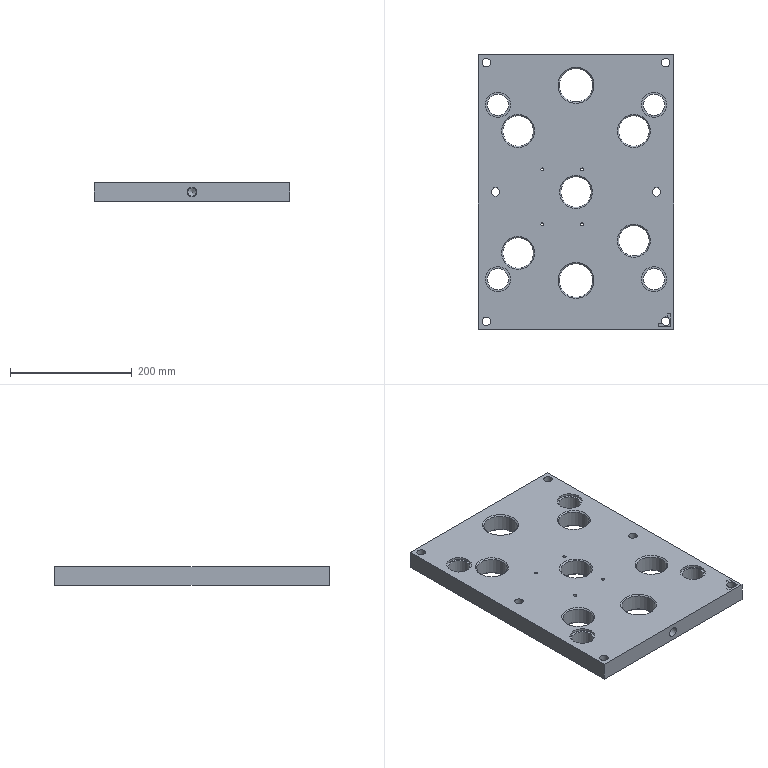Part | STEP file | DZDB | 1 solid | 94 faces | box 320 x 450 x 30 mm | volume 3701626 mm3 | cylinder 41 | plane 31 | cone 22 | commonest cylinder face diameters 6 x6 14 x6 20 x6 50 x5 5 x4 35 x4